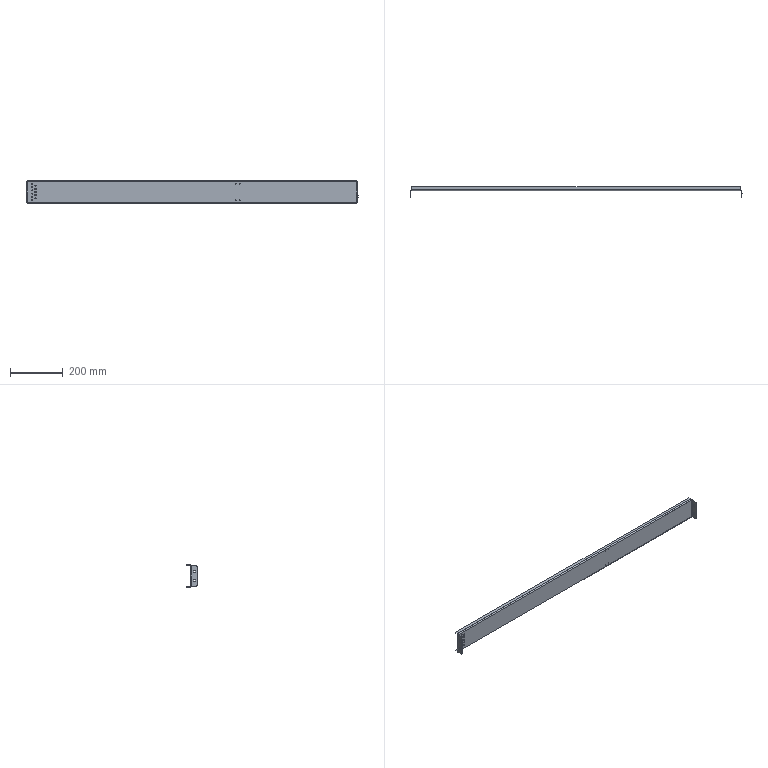Part | SolidWorks | features HoleWzd 4, EdgeFlange 2, Fillet 1, FlatPattern 1, SMBaseFlange 1, SheetMetal 1 | 1 solid | 96 faces | box 1259 x 38 x 85 mm | volume 278401 mm3 | cylinder 58 | plane 38 | commonest cylinder face diameters 4.2 x22 4 x12 5.5 x12 3.3 x8 8 x4